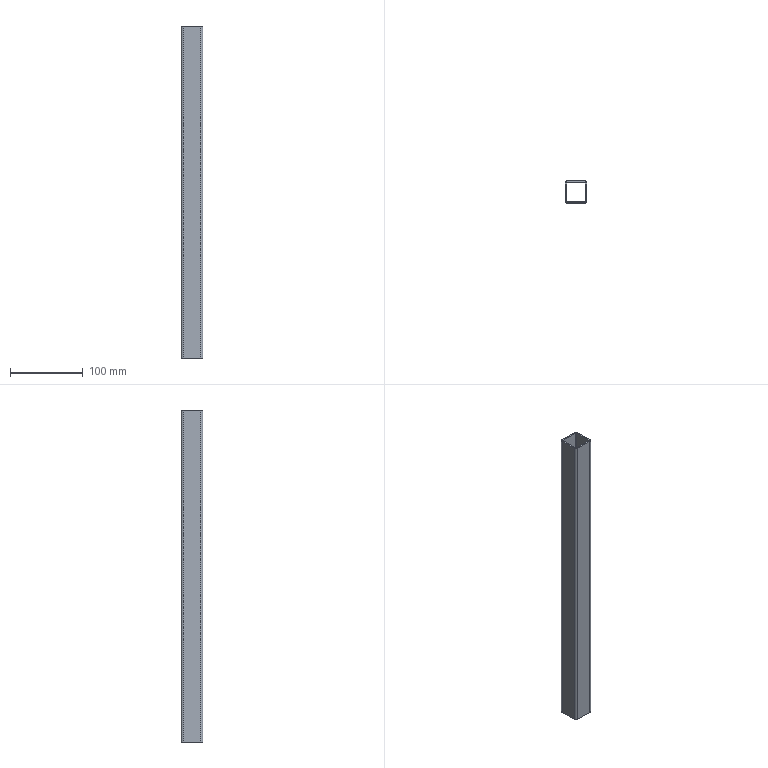Part | STEP file | Leg crossbar 30x30x2 | 1 solid | 18 faces | box 30 x 30 x 456 mm | volume 99013 mm3 | plane 10 | cylinder 8 | commonest cylinder face diameters 2 x4 6 x4
STEP:
#1=CARTESIAN_POINT('',(0.,0.,0.));
#2=DIRECTION('',(0.,0.,1.));
#3=DIRECTION('',(1.,0.,0.));
#4=AXIS2_PLACEMENT_3D('',#1,#2,#3);
#5=CARTESIAN_POINT('',(27.,28.,0.));
#6=VERTEX_POINT('',#5);
#7=CARTESIAN_POINT('',(27.,28.,456.));
#8=VERTEX_POINT('',#7);
#9=CARTESIAN_POINT('',(27.,28.,0.));
#10=DIRECTION('',(0.,0.,1.));
#11=VECTOR('',#10,1.);
#12=LINE('',#9,#11);
#13=CARTESIAN_POINT('',(27.,27.,0.));
#14=DIRECTION('',(0.,0.,1.));
#15=DIRECTION('',(-1.,0.,0.));
#16=AXIS2_PLACEMENT_3D('',#13,#14,#15);
#17=CYLINDRICAL_SURFACE('',#16,1.);
#18=CARTESIAN_POINT('',(4.712,0.));
#19=DIRECTION('',(0.,1.));
#20=VECTOR('',#19,1.);
#21=LINE('',#18,#20);
#22=(GEOMETRIC_REPRESENTATION_CONTEXT(2)PARAMETRIC_REPRESENTATION_CONTEXT()REPRESENTATION_CONTEXT('',''));
#23=DEFINITIONAL_REPRESENTATION('',(#21),#22);
#24=PCURVE('',#17,#23);
#25=CARTESIAN_POINT('',(27.,28.,0.));
#26=DIRECTION('',(0.,1.,0.));
#27=DIRECTION('',(-1.,0.,0.));
#28=AXIS2_PLACEMENT_3D('',#25,#26,#27);
#29=PLANE('',#28);
#30=CARTESIAN_POINT('',(0.,0.));
#31=DIRECTION('',(0.,1.));
#32=VECTOR('',#31,1.);
#33=LINE('',#30,#32);
#34=(GEOMETRIC_REPRESENTATION_CONTEXT(2)PARAMETRIC_REPRESENTATION_CONTEXT()REPRESENTATION_CONTEXT('',''));
#35=DEFINITIONAL_REPRESENTATION('',(#33),#34);
#36=PCURVE('',#29,#35);
#37=SURFACE_CURVE('',#12,(#24,#36),.PCURVE_S1.);
#38=EDGE_CURVE('',#6,#8,#37,.T.);
#39=ORIENTED_EDGE('',*,*,#38,.T.);
#40=CARTESIAN_POINT('',(28.,27.,456.));
#41=VERTEX_POINT('',#40);
#42=CARTESIAN_POINT('',(27.,27.,456.));
#43=DIRECTION('',(0.,0.,-1.));
#44=DIRECTION('',(-1.,0.,0.));
#45=AXIS2_PLACEMENT_3D('',#42,#43,#44);
#46=CIRCLE('',#45,1.);
#47=CARTESIAN_POINT('',(6.283,456.));
#48=DIRECTION('',(-1.,0.));
#49=VECTOR('',#48,1.);
#50=LINE('',#47,#49);
#51=(GEOMETRIC_REPRESENTATION_CONTEXT(2)PARAMETRIC_REPRESENTATION_CONTEXT()REPRESENTATION_CONTEXT('',''));
#52=DEFINITIONAL_REPRESENTATION('',(#50),#51);
#53=PCURVE('',#17,#52);
#54=CARTESIAN_POINT('',(15.,15.,456.));
#55=DIRECTION('',(0.,0.,1.));
#56=DIRECTION('',(1.,0.,0.));
#57=AXIS2_PLACEMENT_3D('',#54,#55,#56);
#58=PLANE('',#57);
#59=CARTESIAN_POINT('',(11.,12.));
#60=CARTESIAN_POINT('',(11.,13.732));
#61=CARTESIAN_POINT('',(12.5,12.866));
#62=CARTESIAN_POINT('',(14.,12.));
#63=CARTESIAN_POINT('',(12.5,11.134));
#64=CARTESIAN_POINT('',(11.,10.268));
#65=CARTESIAN_POINT('',(11.,12.));
#66=(BOUNDED_CURVE()B_SPLINE_CURVE(2,(#59,#60,#61,#62,#63,#64,#65),.UNSPECIFIED.,.T.,.F.)B_SPLINE_CURVE_WITH_KNOTS((1,2,2,2,2,1),(-2.094,0.,2.094,4.189,6.283,8.378),.UNSPECIFIED.)CURVE()GEOMETRIC_REPRESENTATION_ITEM()RATIONAL_B_SPLINE_CURVE((1.,0.5,1.,0.5,1.,0.5,1.))REPRESENTATION_ITEM(''));
#67=(GEOMETRIC_REPRESENTATION_CONTEXT(2)PARAMETRIC_REPRESENTATION_CONTEXT()REPRESENTATION_CONTEXT('',''));
#68=DEFINITIONAL_REPRESENTATION('',(#66),#67);
#69=PCURVE('',#58,#68);
#70=SURFACE_CURVE('',#46,(#53,#69),.PCURVE_S1.);
#71=EDGE_CURVE('',#8,#41,#70,.T.);
#72=ORIENTED_EDGE('',*,*,#71,.T.);
#73=CARTESIAN_POINT('',(28.,27.,0.));
#74=VERTEX_POINT('',#73);
#75=CARTESIAN_POINT('',(28.,27.,0.));
#76=DIRECTION('',(0.,0.,1.));
#77=VECTOR('',#76,1.);
#78=LINE('',#75,#77);
#79=CARTESIAN_POINT('',(3.142,0.));
#80=DIRECTION('',(0.,1.));
#81=VECTOR('',#80,1.);
#82=LINE('',#79,#81);
#83=(GEOMETRIC_REPRESENTATION_CONTEXT(2)PARAMETRIC_REPRESENTATION_CONTEXT()REPRESENTATION_CONTEXT('',''));
#84=DEFINITIONAL_REPRESENTATION('',(#82),#83);
#85=PCURVE('',#17,#84);
#86=CARTESIAN_POINT('',(28.,3.,0.));
#87=DIRECTION('',(1.,0.,0.));
#88=DIRECTION('',(0.,1.,0.));
#89=AXIS2_PLACEMENT_3D('',#86,#87,#88);
#90=PLANE('',#89);
#91=CARTESIAN_POINT('',(24.,0.));
#92=DIRECTION('',(0.,1.));
#93=VECTOR('',#92,1.);
#94=LINE('',#91,#93);
#95=(GEOMETRIC_REPRESENTATION_CONTEXT(2)PARAMETRIC_REPRESENTATION_CONTEXT()REPRESENTATION_CONTEXT('',''));
#96=DEFINITIONAL_REPRESENTATION('',(#94),#95);
#97=PCURVE('',#90,#96);
#98=SURFACE_CURVE('',#78,(#85,#97),.PCURVE_S1.);
#99=EDGE_CURVE('',#74,#41,#98,.T.);
#100=ORIENTED_EDGE('',*,*,#99,.F.);
#101=CARTESIAN_POINT('',(27.,27.,0.));
#102=DIRECTION('',(0.,0.,1.));
#103=DIRECTION('',(-1.,0.,0.));
#104=AXIS2_PLACEMENT_3D('',#101,#102,#103);
#105=CIRCLE('',#104,1.);
#106=CARTESIAN_POINT('',(0.,0.));
#107=DIRECTION('',(1.,0.));
#108=VECTOR('',#107,1.);
#109=LINE('',#106,#108);
#110=(GEOMETRIC_REPRESENTATION_CONTEXT(2)PARAMETRIC_REPRESENTATION_CONTEXT()REPRESENTATION_CONTEXT('',''));
#111=DEFINITIONAL_REPRESENTATION('',(#109),#110);
#112=PCURVE('',#17,#111);
#113=CARTESIAN_POINT('',(15.,15.,0.));
#114=DIRECTION('',(0.,0.,1.));
#115=DIRECTION('',(1.,0.,0.));
#116=AXIS2_PLACEMENT_3D('',#113,#114,#115);
#117=PLANE('',#116);
#118=CARTESIAN_POINT('',(12.,12.));
#119=DIRECTION('',(-1.,0.));
#120=AXIS2_PLACEMENT_2D('',#118,#119);
#121=CIRCLE('',#120,1.);
#122=(GEOMETRIC_REPRESENTATION_CONTEXT(2)PARAMETRIC_REPRESENTATION_CONTEXT()REPRESENTATION_CONTEXT('',''));
#123=DEFINITIONAL_REPRESENTATION('',(#121),#122);
#124=PCURVE('',#117,#123);
#125=SURFACE_CURVE('',#105,(#112,#124),.PCURVE_S1.);
#126=EDGE_CURVE('',#74,#6,#125,.T.);
#127=ORIENTED_EDGE('',*,*,#126,.T.);
#128=EDGE_LOOP('',(#39,#72,#100,#127));
#129=FACE_BOUND('',#128,.F.);
#130=ADVANCED_FACE('',(#129),#17,.F.);
#131=CARTESIAN_POINT('',(28.,3.,0.));
#132=VERTEX_POINT('',#131);
#133=CARTESIAN_POINT('',(28.,9.,0.));
#134=DIRECTION('',(0.,1.,0.));
#135=VECTOR('',#134,1.);
#136=LINE('',#133,#135);
#137=CARTESIAN_POINT('',(6.,0.));
#138=DIRECTION('',(1.,0.));
#139=VECTOR('',#138,1.);
#140=LINE('',#137,#139);
#141=(GEOMETRIC_REPRESENTATION_CONTEXT(2)PARAMETRIC_REPRESENTATION_CONTEXT()REPRESENTATION_CONTEXT('',''));
#142=DEFINITIONAL_REPRESENTATION('',(#140),#141);
#143=PCURVE('',#90,#142);
#144=CARTESIAN_POINT('',(13.,-6.));
#145=DIRECTION('',(0.,1.));
#146=VECTOR('',#145,1.);
#147=LINE('',#144,#146);
#148=(GEOMETRIC_REPRESENTATION_CONTEXT(2)PARAMETRIC_REPRESENTATION_CONTEXT()REPRESENTATION_CONTEXT('',''));
#149=DEFINITIONAL_REPRESENTATION('',(#147),#148);
#150=PCURVE('',#117,#149);
#151=SURFACE_CURVE('',#136,(#143,#150),.PCURVE_S1.);
#152=EDGE_CURVE('',#132,#74,#151,.T.);
#153=ORIENTED_EDGE('',*,*,#152,.F.);
#154=CARTESIAN_POINT('',(28.,3.,456.));
#155=VERTEX_POINT('',#154);
#156=CARTESIAN_POINT('',(28.,3.,0.));
#157=DIRECTION('',(0.,0.,1.));
#158=VECTOR('',#157,1.);
#159=LINE('',#156,#158);
#160=CARTESIAN_POINT('',(0.,0.));
#161=DIRECTION('',(0.,1.));
#162=VECTOR('',#161,1.);
#163=LINE('',#160,#162);
#164=(GEOMETRIC_REPRESENTATION_CONTEXT(2)PARAMETRIC_REPRESENTATION_CONTEXT()REPRESENTATION_CONTEXT('',''));
#165=DEFINITIONAL_REPRESENTATION('',(#163),#164);
#166=PCURVE('',#90,#165);
#167=CARTESIAN_POINT('',(27.,3.,0.));
#168=DIRECTION('',(0.,0.,1.));
#169=DIRECTION('',(0.,1.,0.));
#170=AXIS2_PLACEMENT_3D('',#167,#168,#169);
#171=CYLINDRICAL_SURFACE('',#170,1.);
#172=CARTESIAN_POINT('',(4.712,0.));
#173=DIRECTION('',(0.,1.));
#174=VECTOR('',#173,1.);
#175=LINE('',#172,#174);
#176=(GEOMETRIC_REPRESENTATION_CONTEXT(2)PARAMETRIC_REPRESENTATION_CONTEXT()REPRESENTATION_CONTEXT('',''));
#177=DEFINITIONAL_REPRESENTATION('',(#175),#176);
#178=PCURVE('',#171,#177);
#179=SURFACE_CURVE('',#159,(#166,#178),.PCURVE_S1.);
#180=EDGE_CURVE('',#132,#155,#179,.T.);
#181=ORIENTED_EDGE('',*,*,#180,.T.);
#182=CARTESIAN_POINT('',(28.,9.,456.));
#183=DIRECTION('',(0.,-1.,0.));
#184=VECTOR('',#183,1.);
#185=LINE('',#182,#184);
#186=CARTESIAN_POINT('',(6.,456.));
#187=DIRECTION('',(-1.,0.));
#188=VECTOR('',#187,1.);
#189=LINE('',#186,#188);
#190=(GEOMETRIC_REPRESENTATION_CONTEXT(2)PARAMETRIC_REPRESENTATION_CONTEXT()REPRESENTATION_CONTEXT('',''));
#191=DEFINITIONAL_REPRESENTATION('',(#189),#190);
#192=PCURVE('',#90,#191);
#193=CARTESIAN_POINT('',(13.,-6.));
#194=DIRECTION('',(0.,-1.));
#195=VECTOR('',#194,1.);
#196=LINE('',#193,#195);
#197=(GEOMETRIC_REPRESENTATION_CONTEXT(2)PARAMETRIC_REPRESENTATION_CONTEXT()REPRESENTATION_CONTEXT('',''));
#198=DEFINITIONAL_REPRESENTATION('',(#196),#197);
#199=PCURVE('',#58,#198);
#200=SURFACE_CURVE('',#185,(#192,#199),.PCURVE_S1.);
#201=EDGE_CURVE('',#41,#155,#200,.T.);
#202=ORIENTED_EDGE('',*,*,#201,.F.);
#203=ORIENTED_EDGE('',*,*,#99,.F.);
#204=EDGE_LOOP('',(#153,#181,#202,#203));
#205=FACE_BOUND('',#204,.T.);
#206=ADVANCED_FACE('',(#205),#90,.F.);
#207=ORIENTED_EDGE('',*,*,#180,.T.);
#208=CARTESIAN_POINT('',(27.,2.,456.));
#209=VERTEX_POINT('',#208);
#210=CARTESIAN_POINT('',(27.,3.,456.));
#211=DIRECTION('',(0.,0.,-1.));
#212=DIRECTION('',(0.,1.,0.));
#213=AXIS2_PLACEMENT_3D('',#210,#211,#212);
#214=CIRCLE('',#213,1.);
#215=CARTESIAN_POINT('',(6.283,456.));
#216=DIRECTION('',(-1.,0.));
#217=VECTOR('',#216,1.);
#218=LINE('',#215,#217);
#219=(GEOMETRIC_REPRESENTATION_CONTEXT(2)PARAMETRIC_REPRESENTATION_CONTEXT()REPRESENTATION_CONTEXT('',''));
#220=DEFINITIONAL_REPRESENTATION('',(#218),#219);
#221=PCURVE('',#171,#220);
#222=CARTESIAN_POINT('',(12.,-11.));
#223=CARTESIAN_POINT('',(13.732,-11.));
#224=CARTESIAN_POINT('',(12.866,-12.5));
#225=CARTESIAN_POINT('',(12.,-14.));
#226=CARTESIAN_POINT('',(11.134,-12.5));
#227=CARTESIAN_POINT('',(10.268,-11.));
#228=CARTESIAN_POINT('',(12.,-11.));
#229=(BOUNDED_CURVE()B_SPLINE_CURVE(2,(#222,#223,#224,#225,#226,#227,#228),.UNSPECIFIED.,.T.,.F.)B_SPLINE_CURVE_WITH_KNOTS((1,2,2,2,2,1),(-2.094,0.,2.094,4.189,6.283,8.378),.UNSPECIFIED.)CURVE()GEOMETRIC_REPRESENTATION_ITEM()RATIONAL_B_SPLINE_CURVE((1.,0.5,1.,0.5,1.,0.5,1.))REPRESENTATION_ITEM(''));
#230=(GEOMETRIC_REPRESENTATION_CONTEXT(2)PARAMETRIC_REPRESENTATION_CONTEXT()REPRESENTATION_CONTEXT('',''));
#231=DEFINITIONAL_REPRESENTATION('',(#229),#230);
#232=PCURVE('',#58,#231);
#233=SURFACE_CURVE('',#214,(#221,#232),.PCURVE_S1.);
#234=EDGE_CURVE('',#155,#209,#233,.T.);
#235=ORIENTED_EDGE('',*,*,#234,.T.);
#236=CARTESIAN_POINT('',(27.,2.,0.));
#237=VERTEX_POINT('',#236);
#238=CARTESIAN_POINT('',(27.,2.,0.));
#239=DIRECTION('',(0.,0.,1.));
#240=VECTOR('',#239,1.);
#241=LINE('',#238,#240);
#242=CARTESIAN_POINT('',(3.142,0.));
#243=DIRECTION('',(0.,1.));
#244=VECTOR('',#243,1.);
#245=LINE('',#242,#244);
#246=(GEOMETRIC_REPRESENTATION_CONTEXT(2)PARAMETRIC_REPRESENTATION_CONTEXT()REPRESENTATION_CONTEXT('',''));
#247=DEFINITIONAL_REPRESENTATION('',(#245),#246);
#248=PCURVE('',#171,#247);
#249=CARTESIAN_POINT('',(3.,2.,0.));
#250=DIRECTION('',(0.,-1.,0.));
#251=DIRECTION('',(1.,0.,0.));
#252=AXIS2_PLACEMENT_3D('',#249,#250,#251);
#253=PLANE('',#252);
#254=CARTESIAN_POINT('',(24.,0.));
#255=DIRECTION('',(0.,1.));
#256=VECTOR('',#255,1.);
#257=LINE('',#254,#256);
#258=(GEOMETRIC_REPRESENTATION_CONTEXT(2)PARAMETRIC_REPRESENTATION_CONTEXT()REPRESENTATION_CONTEXT('',''));
#259=DEFINITIONAL_REPRESENTATION('',(#257),#258);
#260=PCURVE('',#253,#259);
#261=SURFACE_CURVE('',#241,(#248,#260),.PCURVE_S1.);
#262=EDGE_CURVE('',#237,#209,#261,.T.);
#263=ORIENTED_EDGE('',*,*,#262,.F.);
#264=CARTESIAN_POINT('',(27.,3.,0.));
#265=DIRECTION('',(0.,0.,1.));
#266=DIRECTION('',(0.,1.,0.));
#267=AXIS2_PLACEMENT_3D('',#264,#265,#266);
#268=CIRCLE('',#267,1.);
#269=CARTESIAN_POINT('',(0.,0.));
#270=DIRECTION('',(1.,0.));
#271=VECTOR('',#270,1.);
#272=LINE('',#269,#271);
#273=(GEOMETRIC_REPRESENTATION_CONTEXT(2)PARAMETRIC_REPRESENTATION_CONTEXT()REPRESENTATION_CONTEXT('',''));
#274=DEFINITIONAL_REPRESENTATION('',(#272),#273);
#275=PCURVE('',#171,#274);
#276=CARTESIAN_POINT('',(12.,-12.));
#277=DIRECTION('',(0.,1.));
#278=AXIS2_PLACEMENT_2D('',#276,#277);
#279=CIRCLE('',#278,1.);
#280=(GEOMETRIC_REPRESENTATION_CONTEXT(2)PARAMETRIC_REPRESENTATION_CONTEXT()REPRESENTATION_CONTEXT('',''));
#281=DEFINITIONAL_REPRESENTATION('',(#279),#280);
#282=PCURVE('',#117,#281);
#283=SURFACE_CURVE('',#268,(#275,#282),.PCURVE_S1.);
#284=EDGE_CURVE('',#237,#132,#283,.T.);
#285=ORIENTED_EDGE('',*,*,#284,.T.);
#286=EDGE_LOOP('',(#207,#235,#263,#285));
#287=FACE_BOUND('',#286,.F.);
#288=ADVANCED_FACE('',(#287),#171,.F.);
#289=CARTESIAN_POINT('',(3.,2.,0.));
#290=VERTEX_POINT('',#289);
#291=CARTESIAN_POINT('',(9.,2.,0.));
#292=DIRECTION('',(1.,0.,0.));
#293=VECTOR('',#292,1.);
#294=LINE('',#291,#293);
#295=CARTESIAN_POINT('',(6.,0.));
#296=DIRECTION('',(1.,0.));
#297=VECTOR('',#296,1.);
#298=LINE('',#295,#297);
#299=(GEOMETRIC_REPRESENTATION_CONTEXT(2)PARAMETRIC_REPRESENTATION_CONTEXT()REPRESENTATION_CONTEXT('',''));
#300=DEFINITIONAL_REPRESENTATION('',(#298),#299);
#301=PCURVE('',#253,#300);
#302=CARTESIAN_POINT('',(-6.,-13.));
#303=DIRECTION('',(1.,0.));
#304=VECTOR('',#303,1.);
#305=LINE('',#302,#304);
#306=(GEOMETRIC_REPRESENTATION_CONTEXT(2)PARAMETRIC_REPRESENTATION_CONTEXT()REPRESENTATION_CONTEXT('',''));
#307=DEFINITIONAL_REPRESENTATION('',(#305),#306);
#308=PCURVE('',#117,#307);
#309=SURFACE_CURVE('',#294,(#301,#308),.PCURVE_S1.);
#310=EDGE_CURVE('',#290,#237,#309,.T.);
#311=ORIENTED_EDGE('',*,*,#310,.F.);
#312=CARTESIAN_POINT('',(3.,2.,456.));
#313=VERTEX_POINT('',#312);
#314=CARTESIAN_POINT('',(3.,2.,0.));
#315=DIRECTION('',(0.,0.,1.));
#316=VECTOR('',#315,1.);
#317=LINE('',#314,#316);
#318=CARTESIAN_POINT('',(0.,0.));
#319=DIRECTION('',(0.,1.));
#320=VECTOR('',#319,1.);
#321=LINE('',#318,#320);
#322=(GEOMETRIC_REPRESENTATION_CONTEXT(2)PARAMETRIC_REPRESENTATION_CONTEXT()REPRESENTATION_CONTEXT('',''));
#323=DEFINITIONAL_REPRESENTATION('',(#321),#322);
#324=PCURVE('',#253,#323);
#325=CARTESIAN_POINT('',(3.,3.,0.));
#326=DIRECTION('',(0.,0.,1.));
#327=DIRECTION('',(1.,0.,0.));
#328=AXIS2_PLACEMENT_3D('',#325,#326,#327);
#329=CYLINDRICAL_SURFACE('',#328,1.);
#330=CARTESIAN_POINT('',(4.712,0.));
#331=DIRECTION('',(0.,1.));
#332=VECTOR('',#331,1.);
#333=LINE('',#330,#332);
#334=(GEOMETRIC_REPRESENTATION_CONTEXT(2)PARAMETRIC_REPRESENTATION_CONTEXT()REPRESENTATION_CONTEXT('',''));
#335=DEFINITIONAL_REPRESENTATION('',(#333),#334);
#336=PCURVE('',#329,#335);
#337=SURFACE_CURVE('',#317,(#324,#336),.PCURVE_S1.);
#338=EDGE_CURVE('',#290,#313,#337,.T.);
#339=ORIENTED_EDGE('',*,*,#338,.T.);
#340=CARTESIAN_POINT('',(9.,2.,456.));
#341=DIRECTION('',(-1.,0.,0.));
#342=VECTOR('',#341,1.);
#343=LINE('',#340,#342);
#344=CARTESIAN_POINT('',(6.,456.));
#345=DIRECTION('',(-1.,0.));
#346=VECTOR('',#345,1.);
#347=LINE('',#344,#346);
#348=(GEOMETRIC_REPRESENTATION_CONTEXT(2)PARAMETRIC_REPRESENTATION_CONTEXT()REPRESENTATION_CONTEXT('',''));
#349=DEFINITIONAL_REPRESENTATION('',(#347),#348);
#350=PCURVE('',#253,#349);
#351=CARTESIAN_POINT('',(-6.,-13.));
#352=DIRECTION('',(-1.,0.));
#353=VECTOR('',#352,1.);
#354=LINE('',#351,#353);
#355=(GEOMETRIC_REPRESENTATION_CONTEXT(2)PARAMETRIC_REPRESENTATION_CONTEXT()REPRESENTATION_CONTEXT('',''));
#356=DEFINITIONAL_REPRESENTATION('',(#354),#355);
#357=PCURVE('',#58,#356);
#358=SURFACE_CURVE('',#343,(#350,#357),.PCURVE_S1.);
#359=EDGE_CURVE('',#209,#313,#358,.T.);
#360=ORIENTED_EDGE('',*,*,#359,.F.);
#361=ORIENTED_EDGE('',*,*,#262,.F.);
#362=EDGE_LOOP('',(#311,#339,#360,#361));
#363=FACE_BOUND('',#362,.T.);
#364=ADVANCED_FACE('',(#363),#253,.F.);
#365=ORIENTED_EDGE('',*,*,#338,.T.);
#366=CARTESIAN_POINT('',(2.,3.,456.));
#367=VERTEX_POINT('',#366);
#368=CARTESIAN_POINT('',(3.,3.,456.));
#369=DIRECTION('',(0.,0.,-1.));
#370=DIRECTION('',(1.,0.,0.));
#371=AXIS2_PLACEMENT_3D('',#368,#369,#370);
#372=CIRCLE('',#371,1.);
#373=CARTESIAN_POINT('',(6.283,456.));
#374=DIRECTION('',(-1.,0.));
#375=VECTOR('',#374,1.);
#376=LINE('',#373,#375);
#377=(GEOMETRIC_REPRESENTATION_CONTEXT(2)PARAMETRIC_REPRESENTATION_CONTEXT()REPRESENTATION_CONTEXT('',''));
#378=DEFINITIONAL_REPRESENTATION('',(#376),#377);
#379=PCURVE('',#329,#378);
#380=CARTESIAN_POINT('',(-11.,-12.));
#381=CARTESIAN_POINT('',(-11.,-13.732));
#382=CARTESIAN_POINT('',(-12.5,-12.866));
#383=CARTESIAN_POINT('',(-14.,-12.));
#384=CARTESIAN_POINT('',(-12.5,-11.134));
#385=CARTESIAN_POINT('',(-11.,-10.268));
#386=CARTESIAN_POINT('',(-11.,-12.));
#387=(BOUNDED_CURVE()B_SPLINE_CURVE(2,(#380,#381,#382,#383,#384,#385,#386),.UNSPECIFIED.,.T.,.F.)B_SPLINE_CURVE_WITH_KNOTS((1,2,2,2,2,1),(-2.094,0.,2.094,4.189,6.283,8.378),.UNSPECIFIED.)CURVE()GEOMETRIC_REPRESENTATION_ITEM()RATIONAL_B_SPLINE_CURVE((1.,0.5,1.,0.5,1.,0.5,1.))REPRESENTATION_ITEM(''));
#388=(GEOMETRIC_REPRESENTATION_CONTEXT(2)PARAMETRIC_REPRESENTATION_CONTEXT()REPRESENTATION_CONTEXT('',''));
#389=DEFINITIONAL_REPRESENTATION('',(#387),#388);
#390=PCURVE('',#58,#389);
#391=SURFACE_CURVE('',#372,(#379,#390),.PCURVE_S1.);
#392=EDGE_CURVE('',#313,#367,#391,.T.);
#393=ORIENTED_EDGE('',*,*,#392,.T.);
#394=CARTESIAN_POINT('',(2.,3.,0.));
#395=VERTEX_POINT('',#394);
#396=CARTESIAN_POINT('',(2.,3.,0.));
#397=DIRECTION('',(0.,0.,1.));
#398=VECTOR('',#397,1.);
#399=LINE('',#396,#398);
#400=CARTESIAN_POINT('',(3.142,0.));
#401=DIRECTION('',(0.,1.));
#402=VECTOR('',#401,1.);
#403=LINE('',#400,#402);
#404=(GEOMETRIC_REPRESENTATION_CONTEXT(2)PARAMETRIC_REPRESENTATION_CONTEXT()REPRESENTATION_CONTEXT('',''));
#405=DEFINITIONAL_REPRESENTATION('',(#403),#404);
#406=PCURVE('',#329,#405);
#407=CARTESIAN_POINT('',(2.,27.,0.));
#408=DIRECTION('',(-1.,0.,0.));
#409=DIRECTION('',(0.,-1.,0.));
#410=AXIS2_PLACEMENT_3D('',#407,#408,#409);
#411=PLANE('',#410);
#412=CARTESIAN_POINT('',(24.,0.));
#413=DIRECTION('',(0.,1.));
#414=VECTOR('',#413,1.);
#415=LINE('',#412,#414);
#416=(GEOMETRIC_REPRESENTATION_CONTEXT(2)PARAMETRIC_REPRESENTATION_CONTEXT()REPRESENTATION_CONTEXT('',''));
#417=DEFINITIONAL_REPRESENTATION('',(#415),#416);
#418=PCURVE('',#411,#417);
#419=SURFACE_CURVE('',#399,(#406,#418),.PCURVE_S1.);
#420=EDGE_CURVE('',#395,#367,#419,.T.);
#421=ORIENTED_EDGE('',*,*,#420,.F.);
#422=CARTESIAN_POINT('',(3.,3.,0.));
#423=DIRECTION('',(0.,0.,1.));
#424=DIRECTION('',(1.,0.,0.));
#425=AXIS2_PLACEMENT_3D('',#422,#423,#424);
#426=CIRCLE('',#425,1.);
#427=CARTESIAN_POINT('',(0.,0.));
#428=DIRECTION('',(1.,0.));
#429=VECTOR('',#428,1.);
#430=LINE('',#427,#429);
#431=(GEOMETRIC_REPRESENTATION_CONTEXT(2)PARAMETRIC_REPRESENTATION_CONTEXT()REPRESENTATION_CONTEXT('',''));
#432=DEFINITIONAL_REPRESENTATION('',(#430),#431);
#433=PCURVE('',#329,#432);
#434=CARTESIAN_POINT('',(-12.,-12.));
#435=DIRECTION('',(1.,0.));
#436=AXIS2_PLACEMENT_2D('',#434,#435);
#437=CIRCLE('',#436,1.);
#438=(GEOMETRIC_REPRESENTATION_CONTEXT(2)PARAMETRIC_REPRESENTATION_CONTEXT()REPRESENTATION_CONTEXT('',''));
#439=DEFINITIONAL_REPRESENTATION('',(#437),#438);
#440=PCURVE('',#117,#439);
#441=SURFACE_CURVE('',#426,(#433,#440),.PCURVE_S1.);
#442=EDGE_CURVE('',#395,#290,#441,.T.);
#443=ORIENTED_EDGE('',*,*,#442,.T.);
#444=EDGE_LOOP('',(#365,#393,#421,#443));
#445=FACE_BOUND('',#444,.F.);
#446=ADVANCED_FACE('',(#445),#329,.F.);
#447=CARTESIAN_POINT('',(2.,27.,0.));
#448=VERTEX_POINT('',#447);
#449=CARTESIAN_POINT('',(2.,21.,0.));
#450=DIRECTION('',(0.,-1.,0.));
#451=VECTOR('',#450,1.);
#452=LINE('',#449,#451);
#453=CARTESIAN_POINT('',(6.,0.));
#454=DIRECTION('',(1.,0.));
#455=VECTOR('',#454,1.);
#456=LINE('',#453,#455);
#457=(GEOMETRIC_REPRESENTATION_CONTEXT(2)PARAMETRIC_REPRESENTATION_CONTEXT()REPRESENTATION_CONTEXT('',''));
#458=DEFINITIONAL_REPRESENTATION('',(#456),#457);
#459=PCURVE('',#411,#458);
#460=CARTESIAN_POINT('',(-13.,6.));
#461=DIRECTION('',(0.,-1.));
#462=VECTOR('',#461,1.);
#463=LINE('',#460,#462);
#464=(GEOMETRIC_REPRESENTATION_CONTEXT(2)PARAMETRIC_REPRESENTATION_CONTEXT()REPRESENTATION_CONTEXT('',''));
#465=DEFINITIONAL_REPRESENTATION('',(#463),#464);
#466=PCURVE('',#117,#465);
#467=SURFACE_CURVE('',#452,(#459,#466),.PCURVE_S1.);
#468=EDGE_CURVE('',#448,#395,#467,.T.);
#469=ORIENTED_EDGE('',*,*,#468,.F.);
#470=CARTESIAN_POINT('',(2.,27.,456.));
#471=VERTEX_POINT('',#470);
#472=CARTESIAN_POINT('',(2.,27.,0.));
#473=DIRECTION('',(0.,0.,1.));
#474=VECTOR('',#473,1.);
#475=LINE('',#472,#474);
#476=CARTESIAN_POINT('',(0.,0.));
#477=DIRECTION('',(0.,1.));
#478=VECTOR('',#477,1.);
#479=LINE('',#476,#478);
#480=(GEOMETRIC_REPRESENTATION_CONTEXT(2)PARAMETRIC_REPRESENTATION_CONTEXT()REPRESENTATION_CONTEXT('',''));
#481=DEFINITIONAL_REPRESENTATION('',(#479),#480);
#482=PCURVE('',#411,#481);
#483=CARTESIAN_POINT('',(3.,27.,0.));
#484=DIRECTION('',(0.,0.,1.));
#485=DIRECTION('',(0.,-1.,0.));
#486=AXIS2_PLACEMENT_3D('',#483,#484,#485);
#487=CYLINDRICAL_SURFACE('',#486,1.);
#488=CARTESIAN_POINT('',(4.712,0.));
#489=DIRECTION('',(0.,1.));
#490=VECTOR('',#489,1.);
#491=LINE('',#488,#490);
#492=(GEOMETRIC_REPRESENTATION_CONTEXT(2)PARAMETRIC_REPRESENTATION_CONTEXT()REPRESENTATION_CONTEXT('',''));
#493=DEFINITIONAL_REPRESENTATION('',(#491),#492);
#494=PCURVE('',#487,#493);
#495=SURFACE_CURVE('',#475,(#482,#494),.PCURVE_S1.);
#496=EDGE_CURVE('',#448,#471,#495,.T.);
#497=ORIENTED_EDGE('',*,*,#496,.T.);
#498=CARTESIAN_POINT('',(2.,21.,456.));
#499=DIRECTION('',(0.,1.,0.));
#500=VECTOR('',#499,1.);
#501=LINE('',#498,#500);
#502=CARTESIAN_POINT('',(6.,456.));
#503=DIRECTION('',(-1.,0.));
#504=VECTOR('',#503,1.);
#505=LINE('',#502,#504);
#506=(GEOMETRIC_REPRESENTATION_CONTEXT(2)PARAMETRIC_REPRESENTATION_CONTEXT()REPRESENTATION_CONTEXT('',''));
#507=DEFINITIONAL_REPRESENTATION('',(#505),#506);
#508=PCURVE('',#411,#507);
#509=CARTESIAN_POINT('',(-13.,6.));
#510=DIRECTION('',(0.,1.));
#511=VECTOR('',#510,1.);
#512=LINE('',#509,#511);
#513=(GEOMETRIC_REPRESENTATION_CONTEXT(2)PARAMETRIC_REPRESENTATION_CONTEXT()REPRESENTATION_CONTEXT('',''));
#514=DEFINITIONAL_REPRESENTATION('',(#512),#513);
#515=PCURVE('',#58,#514);
#516=SURFACE_CURVE('',#501,(#508,#515),.PCURVE_S1.);
#517=EDGE_CURVE('',#367,#471,#516,.T.);
#518=ORIENTED_EDGE('',*,*,#517,.F.);
#519=ORIENTED_EDGE('',*,*,#420,.F.);
#520=EDGE_LOOP('',(#469,#497,#518,#519));
#521=FACE_BOUND('',#520,.T.);
#522=ADVANCED_FACE('',(#521),#411,.F.);
#523=ORIENTED_EDGE('',*,*,#496,.T.);
#524=CARTESIAN_POINT('',(3.,28.,456.));
#525=VERTEX_POINT('',#524);
#526=CARTESIAN_POINT('',(3.,27.,456.));
#527=DIRECTION('',(0.,0.,-1.));
#528=DIRECTION('',(0.,-1.,0.));
#529=AXIS2_PLACEMENT_3D('',#526,#527,#528);
#530=CIRCLE('',#529,1.);
#531=CARTESIAN_POINT('',(6.283,456.));
#532=DIRECTION('',(-1.,0.));
#533=VECTOR('',#532,1.);
#534=LINE('',#531,#533);
#535=(GEOMETRIC_REPRESENTATION_CONTEXT(2)PARAMETRIC_REPRESENTATION_CONTEXT()REPRESENTATION_CONTEXT('',''));
#536=DEFINITIONAL_REPRESENTATION('',(#534),#535);
#537=PCURVE('',#487,#536);
#538=CARTESIAN_POINT('',(-12.,11.));
#539=CARTESIAN_POINT('',(-13.732,11.));
#540=CARTESIAN_POINT('',(-12.866,12.5));
#541=CARTESIAN_POINT('',(-12.,14.));
#542=CARTESIAN_POINT('',(-11.134,12.5));
#543=CARTESIAN_POINT('',(-10.268,11.));
#544=CARTESIAN_POINT('',(-12.,11.));
#545=(BOUNDED_CURVE()B_SPLINE_CURVE(2,(#538,#539,#540,#541,#542,#543,#544),.UNSPECIFIED.,.T.,.F.)B_SPLINE_CURVE_WITH_KNOTS((1,2,2,2,2,1),(-2.094,0.,2.094,4.189,6.283,8.378),.UNSPECIFIED.)CURVE()GEOMETRIC_REPRESENTATION_ITEM()RATIONAL_B_SPLINE_CURVE((1.,0.5,1.,0.5,1.,0.5,1.))REPRESENTATION_ITEM(''));
#546=(GEOMETRIC_REPRESENTATION_CONTEXT(2)PARAMETRIC_REPRESENTATION_CONTEXT()REPRESENTATION_CONTEXT('',''));
#547=DEFINITIONAL_REPRESENTATION('',(#545),#546);
#548=PCURVE('',#58,#547);
#549=SURFACE_CURVE('',#530,(#537,#548),.PCURVE_S1.);
#550=EDGE_CURVE('',#471,#525,#549,.T.);
#551=ORIENTED_EDGE('',*,*,#550,.T.);
#552=CARTESIAN_POINT('',(3.,28.,0.));
#553=VERTEX_POINT('',#552);
#554=CARTESIAN_POINT('',(3.,28.,0.));
#555=DIRECTION('',(0.,0.,1.));
#556=VECTOR('',#555,1.);
#557=LINE('',#554,#556);
#558=CARTESIAN_POINT('',(3.142,0.));
#559=DIRECTION('',(0.,1.));
#560=VECTOR('',#559,1.);
#561=LINE('',#558,#560);
#562=(GEOMETRIC_REPRESENTATION_CONTEXT(2)PARAMETRIC_REPRESENTATION_CONTEXT()REPRESENTATION_CONTEXT('',''));
#563=DEFINITIONAL_REPRESENTATION('',(#561),#562);
#564=PCURVE('',#487,#563);
#565=CARTESIAN_POINT('',(24.,0.));
#566=DIRECTION('',(0.,1.));
#567=VECTOR('',#566,1.);
#568=LINE('',#565,#567);
#569=(GEOMETRIC_REPRESENTATION_CONTEXT(2)PARAMETRIC_REPRESENTATION_CONTEXT()REPRESENTATION_CONTEXT('',''));
#570=DEFINITIONAL_REPRESENTATION('',(#568),#569);
#571=PCURVE('',#29,#570);
#572=SURFACE_CURVE('',#557,(#564,#571),.PCURVE_S1.);
#573=EDGE_CURVE('',#553,#525,#572,.T.);
#574=ORIENTED_EDGE('',*,*,#573,.F.);
#575=CARTESIAN_POINT('',(3.,27.,0.));
#576=DIRECTION('',(0.,0.,1.));
#577=DIRECTION('',(0.,-1.,0.));
#578=AXIS2_PLACEMENT_3D('',#575,#576,#577);
#579=CIRCLE('',#578,1.);
#580=CARTESIAN_POINT('',(0.,0.));
#581=DIRECTION('',(1.,0.));
#582=VECTOR('',#581,1.);
#583=LINE('',#580,#582);
#584=(GEOMETRIC_REPRESENTATION_CONTEXT(2)PARAMETRIC_REPRESENTATION_CONTEXT()REPRESENTATION_CONTEXT('',''));
#585=DEFINITIONAL_REPRESENTATION('',(#583),#584);
#586=PCURVE('',#487,#585);
#587=CARTESIAN_POINT('',(-12.,12.));
#588=DIRECTION('',(0.,-1.));
#589=AXIS2_PLACEMENT_2D('',#587,#588);
#590=CIRCLE('',#589,1.);
#591=(GEOMETRIC_REPRESENTATION_CONTEXT(2)PARAMETRIC_REPRESENTATION_CONTEXT()REPRESENTATION_CONTEXT('',''));
#592=DEFINITIONAL_REPRESENTATION('',(#590),#591);
#593=PCURVE('',#117,#592);
#594=SURFACE_CURVE('',#579,(#586,#593),.PCURVE_S1.);
#595=EDGE_CURVE('',#553,#448,#594,.T.);
#596=ORIENTED_EDGE('',*,*,#595,.T.);
#597=EDGE_LOOP('',(#523,#551,#574,#596));
#598=FACE_BOUND('',#597,.F.);
#599=ADVANCED_FACE('',(#598),#487,.F.);
#600=CARTESIAN_POINT('',(21.,28.,0.));
#601=DIRECTION('',(-1.,0.,0.));
#602=VECTOR('',#601,1.);
#603=LINE('',#600,#602);
#604=CARTESIAN_POINT('',(6.,0.));
#605=DIRECTION('',(1.,0.));
#606=VECTOR('',#605,1.);
#607=LINE('',#604,#606);
#608=(GEOMETRIC_REPRESENTATION_CONTEXT(2)PARAMETRIC_REPRESENTATION_CONTEXT()REPRESENTATION_CONTEXT('',''));
#609=DEFINITIONAL_REPRESENTATION('',(#607),#608);
#610=PCURVE('',#29,#609);
#611=CARTESIAN_POINT('',(6.,13.));
#612=DIRECTION('',(-1.,0.));
#613=VECTOR('',#612,1.);
#614=LINE('',#611,#613);
#615=(GEOMETRIC_REPRESENTATION_CONTEXT(2)PARAMETRIC_REPRESENTATION_CONTEXT()REPRESENTATION_CONTEXT('',''));
#616=DEFINITIONAL_REPRESENTATION('',(#614),#615);
#617=PCURVE('',#117,#616);
#618=SURFACE_CURVE('',#603,(#610,#617),.PCURVE_S1.);
#619=EDGE_CURVE('',#6,#553,#618,.T.);
#620=ORIENTED_EDGE('',*,*,#619,.F.);
#621=ORIENTED_EDGE('',*,*,#38,.T.);
#622=CARTESIAN_POINT('',(21.,28.,456.));
#623=DIRECTION('',(1.,0.,0.));
#624=VECTOR('',#623,1.);
#625=LINE('',#622,#624);
#626=CARTESIAN_POINT('',(6.,456.));
#627=DIRECTION('',(-1.,0.));
#628=VECTOR('',#627,1.);
#629=LINE('',#626,#628);
#630=(GEOMETRIC_REPRESENTATION_CONTEXT(2)PARAMETRIC_REPRESENTATION_CONTEXT()REPRESENTATION_CONTEXT('',''));
#631=DEFINITIONAL_REPRESENTATION('',(#629),#630);
#632=PCURVE('',#29,#631);
#633=CARTESIAN_POINT('',(6.,13.));
#634=DIRECTION('',(1.,0.));
#635=VECTOR('',#634,1.);
#636=LINE('',#633,#635);
#637=(GEOMETRIC_REPRESENTATION_CONTEXT(2)PARAMETRIC_REPRESENTATION_CONTEXT()REPRESENTATION_CONTEXT('',''));
#638=DEFINITIONAL_REPRESENTATION('',(#636),#637);
#639=PCURVE('',#58,#638);
#640=SURFACE_CURVE('',#625,(#632,#639),.PCURVE_S1.);
#641=EDGE_CURVE('',#525,#8,#640,.T.);
#642=ORIENTED_EDGE('',*,*,#641,.F.);
#643=ORIENTED_EDGE('',*,*,#573,.F.);
#644=EDGE_LOOP('',(#620,#621,#642,#643));
#645=FACE_BOUND('',#644,.T.);
#646=ADVANCED_FACE('',(#645),#29,.F.);
#647=CARTESIAN_POINT('',(3.,30.,0.));
#648=VERTEX_POINT('',#647);
#649=CARTESIAN_POINT('',(0.,27.,0.));
#650=VERTEX_POINT('',#649);
#651=CARTESIAN_POINT('',(3.,27.,0.));
#652=DIRECTION('',(0.,0.,1.));
#653=DIRECTION('',(0.,1.,0.));
#654=AXIS2_PLACEMENT_3D('',#651,#652,#653);
#655=CIRCLE('',#654,3.);
#656=CARTESIAN_POINT('',(3.,27.,0.));
#657=DIRECTION('',(0.,0.,1.));
#658=DIRECTION('',(0.,1.,0.));
#659=AXIS2_PLACEMENT_3D('',#656,#657,#658);
#660=CYLINDRICAL_SURFACE('',#659,3.);
#661=CARTESIAN_POINT('',(0.,0.));
#662=DIRECTION('',(1.,0.));
#663=VECTOR('',#662,1.);
#664=LINE('',#661,#663);
#665=(GEOMETRIC_REPRESENTATION_CONTEXT(2)PARAMETRIC_REPRESENTATION_CONTEXT()REPRESENTATION_CONTEXT('',''));
#666=DEFINITIONAL_REPRESENTATION('',(#664),#665);
#667=PCURVE('',#660,#666);
#668=CARTESIAN_POINT('',(-12.,12.));
#669=DIRECTION('',(0.,1.));
#670=AXIS2_PLACEMENT_2D('',#668,#669);
#671=CIRCLE('',#670,3.);
#672=(GEOMETRIC_REPRESENTATION_CONTEXT(2)PARAMETRIC_REPRESENTATION_CONTEXT()REPRESENTATION_CONTEXT('',''));
#673=DEFINITIONAL_REPRESENTATION('',(#671),#672);
#674=PCURVE('',#117,#673);
#675=SURFACE_CURVE('',#655,(#667,#674),.PCURVE_S1.);
#676=EDGE_CURVE('',#648,#650,#675,.T.);
#677=ORIENTED_EDGE('',*,*,#676,.T.);
#678=CARTESIAN_POINT('',(0.,27.,456.));
#679=VERTEX_POINT('',#678);
#680=CARTESIAN_POINT('',(0.,27.,0.));
#681=DIRECTION('',(0.,0.,1.));
#682=VECTOR('',#681,1.);
#683=LINE('',#680,#682);
#684=CARTESIAN_POINT('',(1.571,0.));
#685=DIRECTION('',(0.,1.));
#686=VECTOR('',#685,1.);
#687=LINE('',#684,#686);
#688=(GEOMETRIC_REPRESENTATION_CONTEXT(2)PARAMETRIC_REPRESENTATION_CONTEXT()REPRESENTATION_CONTEXT('',''));
#689=DEFINITIONAL_REPRESENTATION('',(#687),#688);
#690=PCURVE('',#660,#689);
#691=CARTESIAN_POINT('',(0.,27.,0.));
#692=DIRECTION('',(-1.,0.,0.));
#693=DIRECTION('',(0.,-1.,0.));
#694=AXIS2_PLACEMENT_3D('',#691,#692,#693);
#695=PLANE('',#694);
#696=CARTESIAN_POINT('',(0.,0.));
#697=DIRECTION('',(0.,1.));
#698=VECTOR('',#697,1.);
#699=LINE('',#696,#698);
#700=(GEOMETRIC_REPRESENTATION_CONTEXT(2)PARAMETRIC_REPRESENTATION_CONTEXT()REPRESENTATION_CONTEXT('',''));
#701=DEFINITIONAL_REPRESENTATION('',(#699),#700);
#702=PCURVE('',#695,#701);
#703=SURFACE_CURVE('',#683,(#690,#702),.PCURVE_S1.);
#704=EDGE_CURVE('',#650,#679,#703,.T.);
#705=ORIENTED_EDGE('',*,*,#704,.T.);
#706=CARTESIAN_POINT('',(3.,30.,456.));
#707=VERTEX_POINT('',#706);
#708=CARTESIAN_POINT('',(3.,27.,456.));
#709=DIRECTION('',(0.,0.,1.));
#710=DIRECTION('',(0.,1.,0.));
#711=AXIS2_PLACEMENT_3D('',#708,#709,#710);
#712=CIRCLE('',#711,3.);
#713=CARTESIAN_POINT('',(0.,456.));
#714=DIRECTION('',(1.,0.));
#715=VECTOR('',#714,1.);
#716=LINE('',#713,#715);
#717=(GEOMETRIC_REPRESENTATION_CONTEXT(2)PARAMETRIC_REPRESENTATION_CONTEXT()REPRESENTATION_CONTEXT('',''));
#718=DEFINITIONAL_REPRESENTATION('',(#716),#717);
#719=PCURVE('',#660,#718);
#720=CARTESIAN_POINT('',(-12.,12.));
#721=DIRECTION('',(0.,1.));
#722=AXIS2_PLACEMENT_2D('',#720,#721);
#723=CIRCLE('',#722,3.);
#724=(GEOMETRIC_REPRESENTATION_CONTEXT(2)PARAMETRIC_REPRESENTATION_CONTEXT()REPRESENTATION_CONTEXT('',''));
#725=DEFINITIONAL_REPRESENTATION('',(#723),#724);
#726=PCURVE('',#58,#725);
#727=SURFACE_CURVE('',#712,(#719,#726),.PCURVE_S1.);
#728=EDGE_CURVE('',#707,#679,#727,.T.);
#729=ORIENTED_EDGE('',*,*,#728,.F.);
#730=CARTESIAN_POINT('',(3.,30.,0.));
#731=DIRECTION('',(0.,0.,1.));
#732=VECTOR('',#731,1.);
#733=LINE('',#730,#732);
#734=CARTESIAN_POINT('',(0.,0.));
#735=DIRECTION('',(0.,1.));
#736=VECTOR('',#735,1.);
#737=LINE('',#734,#736);
#738=(GEOMETRIC_REPRESENTATION_CONTEXT(2)PARAMETRIC_REPRESENTATION_CONTEXT()REPRESENTATION_CONTEXT('',''));
#739=DEFINITIONAL_REPRESENTATION('',(#737),#738);
#740=PCURVE('',#660,#739);
#741=CARTESIAN_POINT('',(27.,30.,0.));
#742=DIRECTION('',(0.,1.,0.));
#743=DIRECTION('',(-1.,0.,0.));
#744=AXIS2_PLACEMENT_3D('',#741,#742,#743);
#745=PLANE('',#744);
#746=CARTESIAN_POINT('',(24.,0.));
#747=DIRECTION('',(0.,1.));
#748=VECTOR('',#747,1.);
#749=LINE('',#746,#748);
#750=(GEOMETRIC_REPRESENTATION_CONTEXT(2)PARAMETRIC_REPRESENTATION_CONTEXT()REPRESENTATION_CONTEXT('',''));
#751=DEFINITIONAL_REPRESENTATION('',(#749),#750);
#752=PCURVE('',#745,#751);
#753=SURFACE_CURVE('',#733,(#740,#752),.PCURVE_S1.);
#754=EDGE_CURVE('',#648,#707,#753,.T.);
#755=ORIENTED_EDGE('',*,*,#754,.F.);
#756=EDGE_LOOP('',(#677,#705,#729,#755));
#757=FACE_BOUND('',#756,.T.);
#758=ADVANCED_FACE('',(#757),#660,.T.);
#759=CARTESIAN_POINT('',(27.,30.,0.));
#760=VERTEX_POINT('',#759);
#761=CARTESIAN_POINT('',(27.,30.,0.));
#762=DIRECTION('',(-1.,0.,0.));
#763=VECTOR('',#762,1.);
#764=LINE('',#761,#763);
#765=CARTESIAN_POINT('',(0.,0.));
#766=DIRECTION('',(1.,0.));
#767=VECTOR('',#766,1.);
#768=LINE('',#765,#767);
#769=(GEOMETRIC_REPRESENTATION_CONTEXT(2)PARAMETRIC_REPRESENTATION_CONTEXT()REPRESENTATION_CONTEXT('',''));
#770=DEFINITIONAL_REPRESENTATION('',(#768),#769);
#771=PCURVE('',#745,#770);
#772=CARTESIAN_POINT('',(12.,15.));
#773=DIRECTION('',(-1.,0.));
#774=VECTOR('',#773,1.);
#775=LINE('',#772,#774);
#776=(GEOMETRIC_REPRESENTATION_CONTEXT(2)PARAMETRIC_REPRESENTATION_CONTEXT()REPRESENTATION_CONTEXT('',''));
#777=DEFINITIONAL_REPRESENTATION('',(#775),#776);
#778=PCURVE('',#117,#777);
#779=SURFACE_CURVE('',#764,(#771,#778),.PCURVE_S1.);
#780=EDGE_CURVE('',#760,#648,#779,.T.);
#781=ORIENTED_EDGE('',*,*,#780,.T.);
#782=ORIENTED_EDGE('',*,*,#754,.T.);
#783=CARTESIAN_POINT('',(27.,30.,456.));
#784=VERTEX_POINT('',#783);
#785=CARTESIAN_POINT('',(27.,30.,456.));
#786=DIRECTION('',(-1.,0.,0.));
#787=VECTOR('',#786,1.);
#788=LINE('',#785,#787);
#789=CARTESIAN_POINT('',(0.,456.));
#790=DIRECTION('',(1.,0.));
#791=VECTOR('',#790,1.);
#792=LINE('',#789,#791);
#793=(GEOMETRIC_REPRESENTATION_CONTEXT(2)PARAMETRIC_REPRESENTATION_CONTEXT()REPRESENTATION_CONTEXT('',''));
#794=DEFINITIONAL_REPRESENTATION('',(#792),#793);
#795=PCURVE('',#745,#794);
#796=CARTESIAN_POINT('',(12.,15.));
#797=DIRECTION('',(-1.,0.));
#798=VECTOR('',#797,1.);
#799=LINE('',#796,#798);
#800=(GEOMETRIC_REPRESENTATION_CONTEXT(2)PARAMETRIC_REPRESENTATION_CONTEXT()REPRESENTATION_CONTEXT('',''));
#801=DEFINITIONAL_REPRESENTATION('',(#799),#800);
#802=PCURVE('',#58,#801);
#803=SURFACE_CURVE('',#788,(#795,#802),.PCURVE_S1.);
#804=EDGE_CURVE('',#784,#707,#803,.T.);
#805=ORIENTED_EDGE('',*,*,#804,.F.);
#806=CARTESIAN_POINT('',(27.,30.,0.));
#807=DIRECTION('',(0.,0.,1.));
#808=VECTOR('',#807,1.);
#809=LINE('',#806,#808);
#810=CARTESIAN_POINT('',(0.,0.));
#811=DIRECTION('',(0.,1.));
#812=VECTOR('',#811,1.);
#813=LINE('',#810,#812);
#814=(GEOMETRIC_REPRESENTATION_CONTEXT(2)PARAMETRIC_REPRESENTATION_CONTEXT()REPRESENTATION_CONTEXT('',''));
#815=DEFINITIONAL_REPRESENTATION('',(#813),#814);
#816=PCURVE('',#745,#815);
#817=CARTESIAN_POINT('',(27.,27.,0.));
#818=DIRECTION('',(0.,0.,1.));
#819=DIRECTION('',(1.,0.,0.));
#820=AXIS2_PLACEMENT_3D('',#817,#818,#819);
#821=CYLINDRICAL_SURFACE('',#820,3.);
#822=CARTESIAN_POINT('',(1.571,0.));
#823=DIRECTION('',(0.,1.));
#824=VECTOR('',#823,1.);
#825=LINE('',#822,#824);
#826=(GEOMETRIC_REPRESENTATION_CONTEXT(2)PARAMETRIC_REPRESENTATION_CONTEXT()REPRESENTATION_CONTEXT('',''));
#827=DEFINITIONAL_REPRESENTATION('',(#825),#826);
#828=PCURVE('',#821,#827);
#829=SURFACE_CURVE('',#809,(#816,#828),.PCURVE_S1.);
#830=EDGE_CURVE('',#760,#784,#829,.T.);
#831=ORIENTED_EDGE('',*,*,#830,.F.);
#832=EDGE_LOOP('',(#781,#782,#805,#831));
#833=FACE_BOUND('',#832,.T.);
#834=ADVANCED_FACE('',(#833),#745,.T.);
#835=CARTESIAN_POINT('',(30.,27.,0.));
#836=VERTEX_POINT('',#835);
#837=CARTESIAN_POINT('',(27.,27.,0.));
#838=DIRECTION('',(0.,0.,1.));
#839=DIRECTION('',(1.,0.,0.));
#840=AXIS2_PLACEMENT_3D('',#837,#838,#839);
#841=CIRCLE('',#840,3.);
#842=CARTESIAN_POINT('',(0.,0.));
#843=DIRECTION('',(1.,0.));
#844=VECTOR('',#843,1.);
#845=LINE('',#842,#844);
#846=(GEOMETRIC_REPRESENTATION_CONTEXT(2)PARAMETRIC_REPRESENTATION_CONTEXT()REPRESENTATION_CONTEXT('',''));
#847=DEFINITIONAL_REPRESENTATION('',(#845),#846);
#848=PCURVE('',#821,#847);
#849=CARTESIAN_POINT('',(12.,12.));
#850=DIRECTION('',(1.,0.));
#851=AXIS2_PLACEMENT_2D('',#849,#850);
#852=CIRCLE('',#851,3.);
#853=(GEOMETRIC_REPRESENTATION_CONTEXT(2)PARAMETRIC_REPRESENTATION_CONTEXT()REPRESENTATION_CONTEXT('',''));
#854=DEFINITIONAL_REPRESENTATION('',(#852),#853);
#855=PCURVE('',#117,#854);
#856=SURFACE_CURVE('',#841,(#848,#855),.PCURVE_S1.);
#857=EDGE_CURVE('',#836,#760,#856,.T.);
#858=ORIENTED_EDGE('',*,*,#857,.T.);
#859=ORIENTED_EDGE('',*,*,#830,.T.);
#860=CARTESIAN_POINT('',(30.,27.,456.));
#861=VERTEX_POINT('',#860);
#862=CARTESIAN_POINT('',(27.,27.,456.));
#863=DIRECTION('',(0.,0.,1.));
#864=DIRECTION('',(1.,0.,0.));
#865=AXIS2_PLACEMENT_3D('',#862,#863,#864);
#866=CIRCLE('',#865,3.);
#867=CARTESIAN_POINT('',(0.,456.));
#868=DIRECTION('',(1.,0.));
#869=VECTOR('',#868,1.);
#870=LINE('',#867,#869);
#871=(GEOMETRIC_REPRESENTATION_CONTEXT(2)PARAMETRIC_REPRESENTATION_CONTEXT()REPRESENTATION_CONTEXT('',''));
#872=DEFINITIONAL_REPRESENTATION('',(#870),#871);
#873=PCURVE('',#821,#872);
#874=CARTESIAN_POINT('',(12.,12.));
#875=DIRECTION('',(1.,0.));
#876=AXIS2_PLACEMENT_2D('',#874,#875);
#877=CIRCLE('',#876,3.);
#878=(GEOMETRIC_REPRESENTATION_CONTEXT(2)PARAMETRIC_REPRESENTATION_CONTEXT()REPRESENTATION_CONTEXT('',''));
#879=DEFINITIONAL_REPRESENTATION('',(#877),#878);
#880=PCURVE('',#58,#879);
#881=SURFACE_CURVE('',#866,(#873,#880),.PCURVE_S1.);
#882=EDGE_CURVE('',#861,#784,#881,.T.);
#883=ORIENTED_EDGE('',*,*,#882,.F.);
#884=CARTESIAN_POINT('',(30.,27.,0.));
#885=DIRECTION('',(0.,0.,1.));
#886=VECTOR('',#885,1.);
#887=LINE('',#884,#886);
#888=CARTESIAN_POINT('',(0.,0.));
#889=DIRECTION('',(0.,1.));
#890=VECTOR('',#889,1.);
#891=LINE('',#888,#890);
#892=(GEOMETRIC_REPRESENTATION_CONTEXT(2)PARAMETRIC_REPRESENTATION_CONTEXT()REPRESENTATION_CONTEXT('',''));
#893=DEFINITIONAL_REPRESENTATION('',(#891),#892);
#894=PCURVE('',#821,#893);
#895=CARTESIAN_POINT('',(30.,3.,0.));
#896=DIRECTION('',(1.,0.,0.));
#897=DIRECTION('',(0.,1.,0.));
#898=AXIS2_PLACEMENT_3D('',#895,#896,#897);
#899=PLANE('',#898);
#900=CARTESIAN_POINT('',(24.,0.));
#901=DIRECTION('',(0.,1.));
#902=VECTOR('',#901,1.);
#903=LINE('',#900,#902);
#904=(GEOMETRIC_REPRESENTATION_CONTEXT(2)PARAMETRIC_REPRESENTATION_CONTEXT()REPRESENTATION_CONTEXT('',''));
#905=DEFINITIONAL_REPRESENTATION('',(#903),#904);
#906=PCURVE('',#899,#905);
#907=SURFACE_CURVE('',#887,(#894,#906),.PCURVE_S1.);
#908=EDGE_CURVE('',#836,#861,#907,.T.);
#909=ORIENTED_EDGE('',*,*,#908,.F.);
#910=EDGE_LOOP('',(#858,#859,#883,#909));
#911=FACE_BOUND('',#910,.T.);
#912=ADVANCED_FACE('',(#911),#821,.T.);
#913=CARTESIAN_POINT('',(30.,3.,0.));
#914=VERTEX_POINT('',#913);
#915=CARTESIAN_POINT('',(30.,3.,0.));
#916=DIRECTION('',(0.,1.,0.));
#917=VECTOR('',#916,1.);
#918=LINE('',#915,#917);
#919=CARTESIAN_POINT('',(0.,0.));
#920=DIRECTION('',(1.,0.));
#921=VECTOR('',#920,1.);
#922=LINE('',#919,#921);
#923=(GEOMETRIC_REPRESENTATION_CONTEXT(2)PARAMETRIC_REPRESENTATION_CONTEXT()REPRESENTATION_CONTEXT('',''));
#924=DEFINITIONAL_REPRESENTATION('',(#922),#923);
#925=PCURVE('',#899,#924);
#926=CARTESIAN_POINT('',(15.,-12.));
#927=DIRECTION('',(0.,1.));
#928=VECTOR('',#927,1.);
#929=LINE('',#926,#928);
#930=(GEOMETRIC_REPRESENTATION_CONTEXT(2)PARAMETRIC_REPRESENTATION_CONTEXT()REPRESENTATION_CONTEXT('',''));
#931=DEFINITIONAL_REPRESENTATION('',(#929),#930);
#932=PCURVE('',#117,#931);
#933=SURFACE_CURVE('',#918,(#925,#932),.PCURVE_S1.);
#934=EDGE_CURVE('',#914,#836,#933,.T.);
#935=ORIENTED_EDGE('',*,*,#934,.T.);
#936=ORIENTED_EDGE('',*,*,#908,.T.);
#937=CARTESIAN_POINT('',(30.,3.,456.));
#938=VERTEX_POINT('',#937);
#939=CARTESIAN_POINT('',(30.,3.,456.));
#940=DIRECTION('',(0.,1.,0.));
#941=VECTOR('',#940,1.);
#942=LINE('',#939,#941);
#943=CARTESIAN_POINT('',(0.,456.));
#944=DIRECTION('',(1.,0.));
#945=VECTOR('',#944,1.);
#946=LINE('',#943,#945);
#947=(GEOMETRIC_REPRESENTATION_CONTEXT(2)PARAMETRIC_REPRESENTATION_CONTEXT()REPRESENTATION_CONTEXT('',''));
#948=DEFINITIONAL_REPRESENTATION('',(#946),#947);
#949=PCURVE('',#899,#948);
#950=CARTESIAN_POINT('',(15.,-12.));
#951=DIRECTION('',(0.,1.));
#952=VECTOR('',#951,1.);
#953=LINE('',#950,#952);
#954=(GEOMETRIC_REPRESENTATION_CONTEXT(2)PARAMETRIC_REPRESENTATION_CONTEXT()REPRESENTATION_CONTEXT('',''));
#955=DEFINITIONAL_REPRESENTATION('',(#953),#954);
#956=PCURVE('',#58,#955);
#957=SURFACE_CURVE('',#942,(#949,#956),.PCURVE_S1.);
#958=EDGE_CURVE('',#938,#861,#957,.T.);
#959=ORIENTED_EDGE('',*,*,#958,.F.);
#960=CARTESIAN_POINT('',(30.,3.,0.));
#961=DIRECTION('',(0.,0.,1.));
#962=VECTOR('',#961,1.);
#963=LINE('',#960,#962);
#964=CARTESIAN_POINT('',(0.,0.));
#965=DIRECTION('',(0.,1.));
#966=VECTOR('',#965,1.);
#967=LINE('',#964,#966);
#968=(GEOMETRIC_REPRESENTATION_CONTEXT(2)PARAMETRIC_REPRESENTATION_CONTEXT()REPRESENTATION_CONTEXT('',''));
#969=DEFINITIONAL_REPRESENTATION('',(#967),#968);
#970=PCURVE('',#899,#969);
#971=CARTESIAN_POINT('',(27.,3.,0.));
#972=DIRECTION('',(0.,0.,1.));
#973=DIRECTION('',(0.,-1.,0.));
#974=AXIS2_PLACEMENT_3D('',#971,#972,#973);
#975=CYLINDRICAL_SURFACE('',#974,3.);
#976=CARTESIAN_POINT('',(1.571,0.));
#977=DIRECTION('',(0.,1.));
#978=VECTOR('',#977,1.);
#979=LINE('',#976,#978);
#980=(GEOMETRIC_REPRESENTATION_CONTEXT(2)PARAMETRIC_REPRESENTATION_CONTEXT()REPRESENTATION_CONTEXT('',''));
#981=DEFINITIONAL_REPRESENTATION('',(#979),#980);
#982=PCURVE('',#975,#981);
#983=SURFACE_CURVE('',#963,(#970,#982),.PCURVE_S1.);
#984=EDGE_CURVE('',#914,#938,#983,.T.);
#985=ORIENTED_EDGE('',*,*,#984,.F.);
#986=EDGE_LOOP('',(#935,#936,#959,#985));
#987=FACE_BOUND('',#986,.T.);
#988=ADVANCED_FACE('',(#987),#899,.T.);
#989=CARTESIAN_POINT('',(27.,0.,0.));
#990=VERTEX_POINT('',#989);
#991=CARTESIAN_POINT('',(27.,3.,0.));
#992=DIRECTION('',(0.,0.,1.));
#993=DIRECTION('',(0.,-1.,0.));
#994=AXIS2_PLACEMENT_3D('',#991,#992,#993);
#995=CIRCLE('',#994,3.);
#996=CARTESIAN_POINT('',(0.,0.));
#997=DIRECTION('',(1.,0.));
#998=VECTOR('',#997,1.);
#999=LINE('',#996,#998);
#1000=(GEOMETRIC_REPRESENTATION_CONTEXT(2)PARAMETRIC_REPRESENTATION_CONTEXT()REPRESENTATION_CONTEXT('',''));
#1001=DEFINITIONAL_REPRESENTATION('',(#999),#1000);
#1002=PCURVE('',#975,#1001);
#1003=CARTESIAN_POINT('',(12.,-12.));
#1004=DIRECTION('',(0.,-1.));
#1005=AXIS2_PLACEMENT_2D('',#1003,#1004);
#1006=CIRCLE('',#1005,3.);
#1007=(GEOMETRIC_REPRESENTATION_CONTEXT(2)PARAMETRIC_REPRESENTATION_CONTEXT()REPRESENTATION_CONTEXT('',''));
#1008=DEFINITIONAL_REPRESENTATION('',(#1006),#1007);
#1009=PCURVE('',#117,#1008);
#1010=SURFACE_CURVE('',#995,(#1002,#1009),.PCURVE_S1.);
#1011=EDGE_CURVE('',#990,#914,#1010,.T.);
#1012=ORIENTED_EDGE('',*,*,#1011,.T.);
#1013=ORIENTED_EDGE('',*,*,#984,.T.);
#1014=CARTESIAN_POINT('',(27.,0.,456.));
#1015=VERTEX_POINT('',#1014);
#1016=CARTESIAN_POINT('',(27.,3.,456.));
#1017=DIRECTION('',(0.,0.,1.));
#1018=DIRECTION('',(0.,-1.,0.));
#1019=AXIS2_PLACEMENT_3D('',#1016,#1017,#1018);
#1020=CIRCLE('',#1019,3.);
#1021=CARTESIAN_POINT('',(0.,456.));
#1022=DIRECTION('',(1.,0.));
#1023=VECTOR('',#1022,1.);
#1024=LINE('',#1021,#1023);
#1025=(GEOMETRIC_REPRESENTATION_CONTEXT(2)PARAMETRIC_REPRESENTATION_CONTEXT()REPRESENTATION_CONTEXT('',''));
#1026=DEFINITIONAL_REPRESENTATION('',(#1024),#1025);
#1027=PCURVE('',#975,#1026);
#1028=CARTESIAN_POINT('',(12.,-12.));
#1029=DIRECTION('',(0.,-1.));
#1030=AXIS2_PLACEMENT_2D('',#1028,#1029);
#1031=CIRCLE('',#1030,3.);
#1032=(GEOMETRIC_REPRESENTATION_CONTEXT(2)PARAMETRIC_REPRESENTATION_CONTEXT()REPRESENTATION_CONTEXT('',''));
#1033=DEFINITIONAL_REPRESENTATION('',(#1031),#1032);
#1034=PCURVE('',#58,#1033);
#1035=SURFACE_CURVE('',#1020,(#1027,#1034),.PCURVE_S1.);
#1036=EDGE_CURVE('',#1015,#938,#1035,.T.);
#1037=ORIENTED_EDGE('',*,*,#1036,.F.);
#1038=CARTESIAN_POINT('',(27.,0.,0.));
#1039=DIRECTION('',(0.,0.,1.));
#1040=VECTOR('',#1039,1.);
#1041=LINE('',#1038,#1040);
#1042=CARTESIAN_POINT('',(0.,0.));
#1043=DIRECTION('',(0.,1.));
#1044=VECTOR('',#1043,1.);
#1045=LINE('',#1042,#1044);
#1046=(GEOMETRIC_REPRESENTATION_CONTEXT(2)PARAMETRIC_REPRESENTATION_CONTEXT()REPRESENTATION_CONTEXT('',''));
#1047=DEFINITIONAL_REPRESENTATION('',(#1045),#1046);
#1048=PCURVE('',#975,#1047);
#1049=CARTESIAN_POINT('',(3.,0.,0.));
#1050=DIRECTION('',(0.,-1.,0.));
#1051=DIRECTION('',(1.,0.,0.));
#1052=AXIS2_PLACEMENT_3D('',#1049,#1050,#1051);
#1053=PLANE('',#1052);
#1054=CARTESIAN_POINT('',(24.,0.));
#1055=DIRECTION('',(0.,1.));
#1056=VECTOR('',#1055,1.);
#1057=LINE('',#1054,#1056);
#1058=(GEOMETRIC_REPRESENTATION_CONTEXT(2)PARAMETRIC_REPRESENTATION_CONTEXT()REPRESENTATION_CONTEXT('',''));
#1059=DEFINITIONAL_REPRESENTATION('',(#1057),#1058);
#1060=PCURVE('',#1053,#1059);
#1061=SURFACE_CURVE('',#1041,(#1048,#1060),.PCURVE_S1.);
#1062=EDGE_CURVE('',#990,#1015,#1061,.T.);
#1063=ORIENTED_EDGE('',*,*,#1062,.F.);
#1064=EDGE_LOOP('',(#1012,#1013,#1037,#1063));
#1065=FACE_BOUND('',#1064,.T.);
#1066=ADVANCED_FACE('',(#1065),#975,.T.);
#1067=CARTESIAN_POINT('',(3.,0.,0.));
#1068=VERTEX_POINT('',#1067);
#1069=CARTESIAN_POINT('',(3.,0.,0.));
#1070=DIRECTION('',(1.,0.,0.));
#1071=VECTOR('',#1070,1.);
#1072=LINE('',#1069,#1071);
#1073=CARTESIAN_POINT('',(0.,0.));
#1074=DIRECTION('',(1.,0.));
#1075=VECTOR('',#1074,1.);
#1076=LINE('',#1073,#1075);
#1077=(GEOMETRIC_REPRESENTATION_CONTEXT(2)PARAMETRIC_REPRESENTATION_CONTEXT()REPRESENTATION_CONTEXT('',''));
#1078=DEFINITIONAL_REPRESENTATION('',(#1076),#1077);
#1079=PCURVE('',#1053,#1078);
#1080=CARTESIAN_POINT('',(-12.,-15.));
#1081=DIRECTION('',(1.,0.));
#1082=VECTOR('',#1081,1.);
#1083=LINE('',#1080,#1082);
#1084=(GEOMETRIC_REPRESENTATION_CONTEXT(2)PARAMETRIC_REPRESENTATION_CONTEXT()REPRESENTATION_CONTEXT('',''));
#1085=DEFINITIONAL_REPRESENTATION('',(#1083),#1084);
#1086=PCURVE('',#117,#1085);
#1087=SURFACE_CURVE('',#1072,(#1079,#1086),.PCURVE_S1.);
#1088=EDGE_CURVE('',#1068,#990,#1087,.T.);
#1089=ORIENTED_EDGE('',*,*,#1088,.T.);
#1090=ORIENTED_EDGE('',*,*,#1062,.T.);
#1091=CARTESIAN_POINT('',(3.,0.,456.));
#1092=VERTEX_POINT('',#1091);
#1093=CARTESIAN_POINT('',(3.,0.,456.));
#1094=DIRECTION('',(1.,0.,0.));
#1095=VECTOR('',#1094,1.);
#1096=LINE('',#1093,#1095);
#1097=CARTESIAN_POINT('',(0.,456.));
#1098=DIRECTION('',(1.,0.));
#1099=VECTOR('',#1098,1.);
#1100=LINE('',#1097,#1099);
#1101=(GEOMETRIC_REPRESENTATION_CONTEXT(2)PARAMETRIC_REPRESENTATION_CONTEXT()REPRESENTATION_CONTEXT('',''));
#1102=DEFINITIONAL_REPRESENTATION('',(#1100),#1101);
#1103=PCURVE('',#1053,#1102);
#1104=CARTESIAN_POINT('',(-12.,-15.));
#1105=DIRECTION('',(1.,0.));
#1106=VECTOR('',#1105,1.);
#1107=LINE('',#1104,#1106);
#1108=(GEOMETRIC_REPRESENTATION_CONTEXT(2)PARAMETRIC_REPRESENTATION_CONTEXT()REPRESENTATION_CONTEXT('',''));
#1109=DEFINITIONAL_REPRESENTATION('',(#1107),#1108);
#1110=PCURVE('',#58,#1109);
#1111=SURFACE_CURVE('',#1096,(#1103,#1110),.PCURVE_S1.);
#1112=EDGE_CURVE('',#1092,#1015,#1111,.T.);
#1113=ORIENTED_EDGE('',*,*,#1112,.F.);
#1114=CARTESIAN_POINT('',(3.,0.,0.));
#1115=DIRECTION('',(0.,0.,1.));
#1116=VECTOR('',#1115,1.);
#1117=LINE('',#1114,#1116);
#1118=CARTESIAN_POINT('',(0.,0.));
#1119=DIRECTION('',(0.,1.));
#1120=VECTOR('',#1119,1.);
#1121=LINE('',#1118,#1120);
#1122=(GEOMETRIC_REPRESENTATION_CONTEXT(2)PARAMETRIC_REPRESENTATION_CONTEXT()REPRESENTATION_CONTEXT('',''));
#1123=DEFINITIONAL_REPRESENTATION('',(#1121),#1122);
#1124=PCURVE('',#1053,#1123);
#1125=CARTESIAN_POINT('',(3.,3.,0.));
#1126=DIRECTION('',(0.,0.,1.));
#1127=DIRECTION('',(-1.,0.,0.));
#1128=AXIS2_PLACEMENT_3D('',#1125,#1126,#1127);
#1129=CYLINDRICAL_SURFACE('',#1128,3.);
#1130=CARTESIAN_POINT('',(1.571,0.));
#1131=DIRECTION('',(0.,1.));
#1132=VECTOR('',#1131,1.);
#1133=LINE('',#1130,#1132);
#1134=(GEOMETRIC_REPRESENTATION_CONTEXT(2)PARAMETRIC_REPRESENTATION_CONTEXT()REPRESENTATION_CONTEXT('',''));
#1135=DEFINITIONAL_REPRESENTATION('',(#1133),#1134);
#1136=PCURVE('',#1129,#1135);
#1137=SURFACE_CURVE('',#1117,(#1124,#1136),.PCURVE_S1.);
#1138=EDGE_CURVE('',#1068,#1092,#1137,.T.);
#1139=ORIENTED_EDGE('',*,*,#1138,.F.);
#1140=EDGE_LOOP('',(#1089,#1090,#1113,#1139));
#1141=FACE_BOUND('',#1140,.T.);
#1142=ADVANCED_FACE('',(#1141),#1053,.T.);
#1143=CARTESIAN_POINT('',(0.,3.,0.));
#1144=VERTEX_POINT('',#1143);
#1145=CARTESIAN_POINT('',(3.,3.,0.));
#1146=DIRECTION('',(0.,0.,1.));
#1147=DIRECTION('',(-1.,0.,0.));
#1148=AXIS2_PLACEMENT_3D('',#1145,#1146,#1147);
#1149=CIRCLE('',#1148,3.);
#1150=CARTESIAN_POINT('',(0.,0.));
#1151=DIRECTION('',(1.,0.));
#1152=VECTOR('',#1151,1.);
#1153=LINE('',#1150,#1152);
#1154=(GEOMETRIC_REPRESENTATION_CONTEXT(2)PARAMETRIC_REPRESENTATION_CONTEXT()REPRESENTATION_CONTEXT('',''));
#1155=DEFINITIONAL_REPRESENTATION('',(#1153),#1154);
#1156=PCURVE('',#1129,#1155);
#1157=CARTESIAN_POINT('',(-12.,-12.));
#1158=DIRECTION('',(-1.,0.));
#1159=AXIS2_PLACEMENT_2D('',#1157,#1158);
#1160=CIRCLE('',#1159,3.);
#1161=(GEOMETRIC_REPRESENTATION_CONTEXT(2)PARAMETRIC_REPRESENTATION_CONTEXT()REPRESENTATION_CONTEXT('',''));
#1162=DEFINITIONAL_REPRESENTATION('',(#1160),#1161);
#1163=PCURVE('',#117,#1162);
#1164=SURFACE_CURVE('',#1149,(#1156,#1163),.PCURVE_S1.);
#1165=EDGE_CURVE('',#1144,#1068,#1164,.T.);
#1166=ORIENTED_EDGE('',*,*,#1165,.T.);
#1167=ORIENTED_EDGE('',*,*,#1138,.T.);
#1168=CARTESIAN_POINT('',(0.,3.,456.));
#1169=VERTEX_POINT('',#1168);
#1170=CARTESIAN_POINT('',(3.,3.,456.));
#1171=DIRECTION('',(0.,0.,1.));
#1172=DIRECTION('',(-1.,0.,0.));
#1173=AXIS2_PLACEMENT_3D('',#1170,#1171,#1172);
#1174=CIRCLE('',#1173,3.);
#1175=CARTESIAN_POINT('',(0.,456.));
#1176=DIRECTION('',(1.,0.));
#1177=VECTOR('',#1176,1.);
#1178=LINE('',#1175,#1177);
#1179=(GEOMETRIC_REPRESENTATION_CONTEXT(2)PARAMETRIC_REPRESENTATION_CONTEXT()REPRESENTATION_CONTEXT('',''));
#1180=DEFINITIONAL_REPRESENTATION('',(#1178),#1179);
#1181=PCURVE('',#1129,#1180);
#1182=CARTESIAN_POINT('',(-12.,-12.));
#1183=DIRECTION('',(-1.,0.));
#1184=AXIS2_PLACEMENT_2D('',#1182,#1183);
#1185=CIRCLE('',#1184,3.);
#1186=(GEOMETRIC_REPRESENTATION_CONTEXT(2)PARAMETRIC_REPRESENTATION_CONTEXT()REPRESENTATION_CONTEXT('',''));
#1187=DEFINITIONAL_REPRESENTATION('',(#1185),#1186);
#1188=PCURVE('',#58,#1187);
#1189=SURFACE_CURVE('',#1174,(#1181,#1188),.PCURVE_S1.);
#1190=EDGE_CURVE('',#1169,#1092,#1189,.T.);
#1191=ORIENTED_EDGE('',*,*,#1190,.F.);
#1192=CARTESIAN_POINT('',(0.,3.,0.));
#1193=DIRECTION('',(0.,0.,1.));
#1194=VECTOR('',#1193,1.);
#1195=LINE('',#1192,#1194);
#1196=CARTESIAN_POINT('',(0.,0.));
#1197=DIRECTION('',(0.,1.));
#1198=VECTOR('',#1197,1.);
#1199=LINE('',#1196,#1198);
#1200=(GEOMETRIC_REPRESENTATION_CONTEXT(2)PARAMETRIC_REPRESENTATION_CONTEXT()REPRESENTATION_CONTEXT('',''));
#1201=DEFINITIONAL_REPRESENTATION('',(#1199),#1200);
#1202=PCURVE('',#1129,#1201);
#1203=CARTESIAN_POINT('',(24.,0.));
#1204=DIRECTION('',(0.,1.));
#1205=VECTOR('',#1204,1.);
#1206=LINE('',#1203,#1205);
#1207=(GEOMETRIC_REPRESENTATION_CONTEXT(2)PARAMETRIC_REPRESENTATION_CONTEXT()REPRESENTATION_CONTEXT('',''));
#1208=DEFINITIONAL_REPRESENTATION('',(#1206),#1207);
#1209=PCURVE('',#695,#1208);
#1210=SURFACE_CURVE('',#1195,(#1202,#1209),.PCURVE_S1.);
#1211=EDGE_CURVE('',#1144,#1169,#1210,.T.);
#1212=ORIENTED_EDGE('',*,*,#1211,.F.);
#1213=EDGE_LOOP('',(#1166,#1167,#1191,#1212));
#1214=FACE_BOUND('',#1213,.T.);
#1215=ADVANCED_FACE('',(#1214),#1129,.T.);
#1216=CARTESIAN_POINT('',(0.,27.,0.));
#1217=DIRECTION('',(0.,-1.,0.));
#1218=VECTOR('',#1217,1.);
#1219=LINE('',#1216,#1218);
#1220=CARTESIAN_POINT('',(0.,0.));
#1221=DIRECTION('',(1.,0.));
#1222=VECTOR('',#1221,1.);
#1223=LINE('',#1220,#1222);
#1224=(GEOMETRIC_REPRESENTATION_CONTEXT(2)PARAMETRIC_REPRESENTATION_CONTEXT()REPRESENTATION_CONTEXT('',''));
#1225=DEFINITIONAL_REPRESENTATION('',(#1223),#1224);
#1226=PCURVE('',#695,#1225);
#1227=CARTESIAN_POINT('',(-15.,12.));
#1228=DIRECTION('',(0.,-1.));
#1229=VECTOR('',#1228,1.);
#1230=LINE('',#1227,#1229);
#1231=(GEOMETRIC_REPRESENTATION_CONTEXT(2)PARAMETRIC_REPRESENTATION_CONTEXT()REPRESENTATION_CONTEXT('',''));
#1232=DEFINITIONAL_REPRESENTATION('',(#1230),#1231);
#1233=PCURVE('',#117,#1232);
#1234=SURFACE_CURVE('',#1219,(#1226,#1233),.PCURVE_S1.);
#1235=EDGE_CURVE('',#650,#1144,#1234,.T.);
#1236=ORIENTED_EDGE('',*,*,#1235,.T.);
#1237=ORIENTED_EDGE('',*,*,#1211,.T.);
#1238=CARTESIAN_POINT('',(0.,27.,456.));
#1239=DIRECTION('',(0.,-1.,0.));
#1240=VECTOR('',#1239,1.);
#1241=LINE('',#1238,#1240);
#1242=CARTESIAN_POINT('',(0.,456.));
#1243=DIRECTION('',(1.,0.));
#1244=VECTOR('',#1243,1.);
#1245=LINE('',#1242,#1244);
#1246=(GEOMETRIC_REPRESENTATION_CONTEXT(2)PARAMETRIC_REPRESENTATION_CONTEXT()REPRESENTATION_CONTEXT('',''));
#1247=DEFINITIONAL_REPRESENTATION('',(#1245),#1246);
#1248=PCURVE('',#695,#1247);
#1249=CARTESIAN_POINT('',(-15.,12.));
#1250=DIRECTION('',(0.,-1.));
#1251=VECTOR('',#1250,1.);
#1252=LINE('',#1249,#1251);
#1253=(GEOMETRIC_REPRESENTATION_CONTEXT(2)PARAMETRIC_REPRESENTATION_CONTEXT()REPRESENTATION_CONTEXT('',''));
#1254=DEFINITIONAL_REPRESENTATION('',(#1252),#1253);
#1255=PCURVE('',#58,#1254);
#1256=SURFACE_CURVE('',#1241,(#1248,#1255),.PCURVE_S1.);
#1257=EDGE_CURVE('',#679,#1169,#1256,.T.);
#1258=ORIENTED_EDGE('',*,*,#1257,.F.);
#1259=ORIENTED_EDGE('',*,*,#704,.F.);
#1260=EDGE_LOOP('',(#1236,#1237,#1258,#1259));
#1261=FACE_BOUND('',#1260,.T.);
#1262=ADVANCED_FACE('',(#1261),#695,.T.);
#1263=ORIENTED_EDGE('',*,*,#1257,.T.);
#1264=ORIENTED_EDGE('',*,*,#1190,.T.);
#1265=ORIENTED_EDGE('',*,*,#1112,.T.);
#1266=ORIENTED_EDGE('',*,*,#1036,.T.);
#1267=ORIENTED_EDGE('',*,*,#958,.T.);
#1268=ORIENTED_EDGE('',*,*,#882,.T.);
#1269=ORIENTED_EDGE('',*,*,#804,.T.);
#1270=ORIENTED_EDGE('',*,*,#728,.T.);
#1271=EDGE_LOOP('',(#1263,#1264,#1265,#1266,#1267,#1268,#1269,#1270));
#1272=FACE_BOUND('',#1271,.T.);
#1273=ORIENTED_EDGE('',*,*,#71,.T.);
#1274=ORIENTED_EDGE('',*,*,#201,.T.);
#1275=ORIENTED_EDGE('',*,*,#234,.T.);
#1276=ORIENTED_EDGE('',*,*,#359,.T.);
#1277=ORIENTED_EDGE('',*,*,#392,.T.);
#1278=ORIENTED_EDGE('',*,*,#517,.T.);
#1279=ORIENTED_EDGE('',*,*,#550,.T.);
#1280=ORIENTED_EDGE('',*,*,#641,.T.);
#1281=EDGE_LOOP('',(#1273,#1274,#1275,#1276,#1277,#1278,#1279,#1280));
#1282=FACE_BOUND('',#1281,.T.);
#1283=ADVANCED_FACE('',(#1272,#1282),#58,.T.);
#1284=ORIENTED_EDGE('',*,*,#1235,.F.);
#1285=ORIENTED_EDGE('',*,*,#676,.F.);
#1286=ORIENTED_EDGE('',*,*,#780,.F.);
#1287=ORIENTED_EDGE('',*,*,#857,.F.);
#1288=ORIENTED_EDGE('',*,*,#934,.F.);
#1289=ORIENTED_EDGE('',*,*,#1011,.F.);
#1290=ORIENTED_EDGE('',*,*,#1088,.F.);
#1291=ORIENTED_EDGE('',*,*,#1165,.F.);
#1292=EDGE_LOOP('',(#1284,#1285,#1286,#1287,#1288,#1289,#1290,#1291));
#1293=FACE_BOUND('',#1292,.T.);
#1294=ORIENTED_EDGE('',*,*,#126,.T.);
#1295=ORIENTED_EDGE('',*,*,#619,.T.);
#1296=ORIENTED_EDGE('',*,*,#595,.T.);
#1297=ORIENTED_EDGE('',*,*,#468,.T.);
#1298=ORIENTED_EDGE('',*,*,#442,.T.);
#1299=ORIENTED_EDGE('',*,*,#310,.T.);
#1300=ORIENTED_EDGE('',*,*,#284,.T.);
#1301=ORIENTED_EDGE('',*,*,#152,.T.);
#1302=EDGE_LOOP('',(#1294,#1295,#1296,#1297,#1298,#1299,#1300,#1301));
#1303=FACE_BOUND('',#1302,.T.);
#1304=ADVANCED_FACE('',(#1293,#1303),#117,.F.);
#1305=CLOSED_SHELL('',(#130,#206,#288,#364,#446,#522,#599,#646,#758,#834,#912,#988,#1066,#1142,#1215,#1262,#1283,#1304));
#1306=MANIFOLD_SOLID_BREP('',#1305);
#1307=(LENGTH_UNIT()NAMED_UNIT(*)SI_UNIT(.MILLI.,.METRE.));
#1308=UNCERTAINTY_MEASURE_WITH_UNIT(LENGTH_MEASURE(0.0000001),#1307,'','');
#1309=(NAMED_UNIT(*)PLANE_ANGLE_UNIT()SI_UNIT($,.RADIAN.));
#1310=(NAMED_UNIT(*)SI_UNIT($,.STERADIAN.)SOLID_ANGLE_UNIT());
#1311=(GEOMETRIC_REPRESENTATION_CONTEXT(3)GLOBAL_UNCERTAINTY_ASSIGNED_CONTEXT((#1308))GLOBAL_UNIT_ASSIGNED_CONTEXT((#1307,#1309,#1310))REPRESENTATION_CONTEXT('',''));
#1312=ADVANCED_BREP_SHAPE_REPRESENTATION('',(#4,#1306),#1311);